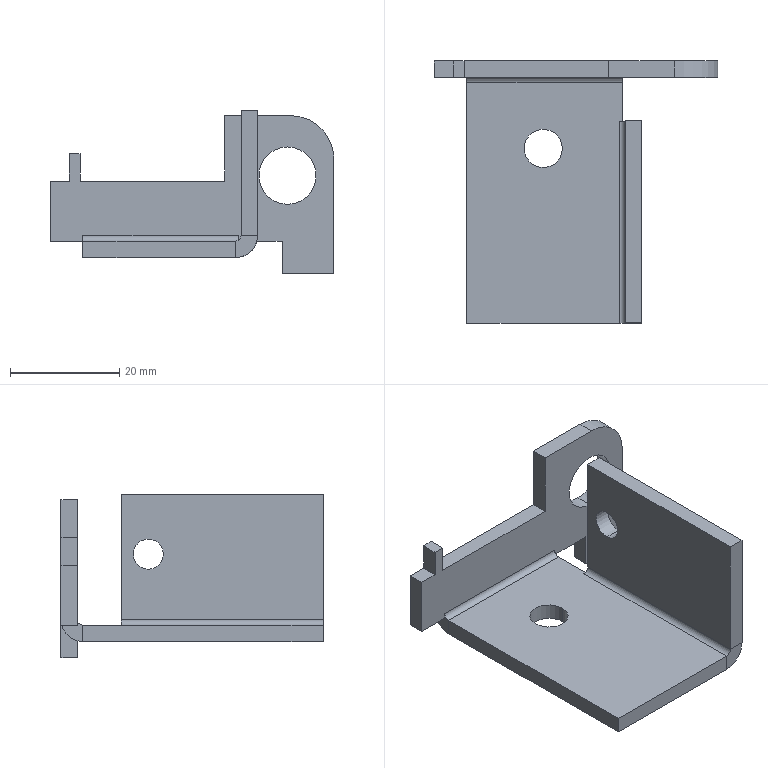Part | STEP file | 8XS123012 | 1 solid | 43 faces | box 52 x 48 x 30 mm | volume 9095 mm3 | plane 32 | cylinder 11 | commonest cylinder face diameters 2 x2 5.5 x2 7 x2 8 x2 10.5 x2 16 x1